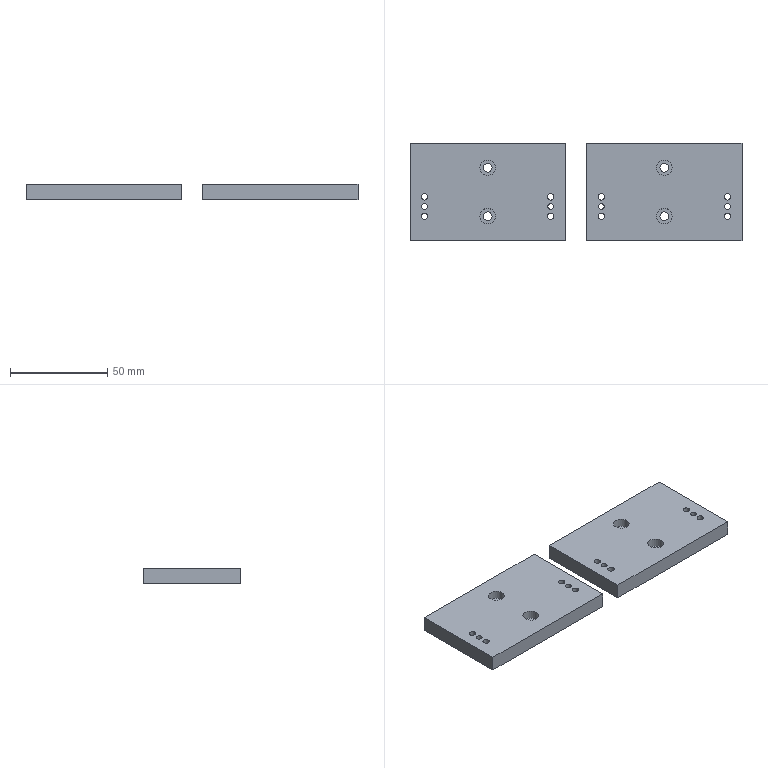Part | NX | 2 solids | 44 faces | box 171 x 50 x 8 mm | volume 62014 mm3 | cylinder 24 | plane 20 | commonest cylinder face diameters 3.3 x8 3 x4 4.5 x4 6 x4 8 x4
STEP:
#1=CARTESIAN_POINT('',(93.25,12.5,2.));
#2=VERTEX_POINT('',#1);
#3=CARTESIAN_POINT('',(91.,12.5,2.));
#4=DIRECTION('',(0.,0.,-1.));
#5=DIRECTION('',(1.,0.,0.));
#6=AXIS2_PLACEMENT_3D('',#3,#4,#5);
#7=CIRCLE('',#6,2.25);
#8=EDGE_CURVE('',#2,#2,#7,.T.);
#9=ORIENTED_EDGE('',*,*,#8,.F.);
#10=EDGE_LOOP('',(#9));
#11=FACE_BOUND('',#10,.T.);
#12=CARTESIAN_POINT('',(94.,12.5,2.));
#13=VERTEX_POINT('',#12);
#14=CARTESIAN_POINT('',(91.,12.5,2.));
#15=DIRECTION('',(0.,0.,-1.));
#16=DIRECTION('',(1.,0.,0.));
#17=AXIS2_PLACEMENT_3D('',#14,#15,#16);
#18=CIRCLE('',#17,3.);
#19=EDGE_CURVE('',#13,#13,#18,.T.);
#20=ORIENTED_EDGE('',*,*,#19,.T.);
#21=EDGE_LOOP('',(#20));
#22=FACE_BOUND('',#21,.T.);
#23=CARTESIAN_POINT('',(91.,37.5,2.));
#24=DIRECTION('',(0.,0.,1.));
#25=DIRECTION('',(1.,0.,0.));
#26=AXIS2_PLACEMENT_3D('',#23,#24,#25);
#27=PLANE('',#26);
#28=ADVANCED_FACE('',(#11,#22),#27,.F.);
#29=CARTESIAN_POINT('',(93.25,37.5,2.));
#30=VERTEX_POINT('',#29);
#31=CARTESIAN_POINT('',(91.,37.5,2.));
#32=DIRECTION('',(0.,0.,-1.));
#33=DIRECTION('',(1.,0.,0.));
#34=AXIS2_PLACEMENT_3D('',#31,#32,#33);
#35=CIRCLE('',#34,2.25);
#36=EDGE_CURVE('',#30,#30,#35,.T.);
#37=ORIENTED_EDGE('',*,*,#36,.F.);
#38=EDGE_LOOP('',(#37));
#39=FACE_BOUND('',#38,.T.);
#40=CARTESIAN_POINT('',(88.,37.5,2.));
#41=VERTEX_POINT('',#40);
#42=CARTESIAN_POINT('',(91.,37.5,2.));
#43=DIRECTION('',(0.,0.,-1.));
#44=DIRECTION('',(-1.,0.,0.));
#45=AXIS2_PLACEMENT_3D('',#42,#43,#44);
#46=CIRCLE('',#45,3.);
#47=EDGE_CURVE('',#41,#41,#46,.T.);
#48=ORIENTED_EDGE('',*,*,#47,.T.);
#49=EDGE_LOOP('',(#48));
#50=FACE_BOUND('',#49,.T.);
#51=CARTESIAN_POINT('',(91.,37.5,2.));
#52=DIRECTION('',(0.,0.,1.));
#53=DIRECTION('',(1.,0.,0.));
#54=AXIS2_PLACEMENT_3D('',#51,#52,#53);
#55=PLANE('',#54);
#56=ADVANCED_FACE('',(#39,#50),#55,.F.);
#57=CARTESIAN_POINT('',(95.,37.5,3.6));
#58=VERTEX_POINT('',#57);
#59=CARTESIAN_POINT('',(91.,37.5,3.6));
#60=DIRECTION('',(0.,0.,1.));
#61=DIRECTION('',(1.,0.,0.));
#62=AXIS2_PLACEMENT_3D('',#59,#60,#61);
#63=CIRCLE('',#62,4.);
#64=EDGE_CURVE('',#58,#58,#63,.T.);
#65=ORIENTED_EDGE('',*,*,#64,.T.);
#66=EDGE_LOOP('',(#65));
#67=FACE_BOUND('',#66,.T.);
#68=CARTESIAN_POINT('',(93.25,37.5,3.6));
#69=VERTEX_POINT('',#68);
#70=CARTESIAN_POINT('',(91.,37.5,3.6));
#71=DIRECTION('',(0.,0.,1.));
#72=DIRECTION('',(1.,0.,0.));
#73=AXIS2_PLACEMENT_3D('',#70,#71,#72);
#74=CIRCLE('',#73,2.25);
#75=EDGE_CURVE('',#69,#69,#74,.T.);
#76=ORIENTED_EDGE('',*,*,#75,.F.);
#77=EDGE_LOOP('',(#76));
#78=FACE_BOUND('',#77,.T.);
#79=CARTESIAN_POINT('',(93.25,37.5,3.6));
#80=DIRECTION('',(0.,0.,-1.));
#81=DIRECTION('',(-1.,0.,0.));
#82=AXIS2_PLACEMENT_3D('',#79,#80,#81);
#83=PLANE('',#82);
#84=ADVANCED_FACE('',(#67,#78),#83,.F.);
#85=CARTESIAN_POINT('',(87.,12.5,3.6));
#86=VERTEX_POINT('',#85);
#87=CARTESIAN_POINT('',(91.,12.5,3.6));
#88=DIRECTION('',(0.,0.,1.));
#89=DIRECTION('',(-1.,0.,0.));
#90=AXIS2_PLACEMENT_3D('',#87,#88,#89);
#91=CIRCLE('',#90,4.);
#92=EDGE_CURVE('',#86,#86,#91,.T.);
#93=ORIENTED_EDGE('',*,*,#92,.T.);
#94=EDGE_LOOP('',(#93));
#95=FACE_BOUND('',#94,.T.);
#96=CARTESIAN_POINT('',(88.75,12.5,3.6));
#97=VERTEX_POINT('',#96);
#98=CARTESIAN_POINT('',(91.,12.5,3.6));
#99=DIRECTION('',(0.,0.,1.));
#100=DIRECTION('',(-1.,0.,0.));
#101=AXIS2_PLACEMENT_3D('',#98,#99,#100);
#102=CIRCLE('',#101,2.25);
#103=EDGE_CURVE('',#97,#97,#102,.T.);
#104=ORIENTED_EDGE('',*,*,#103,.F.);
#105=EDGE_LOOP('',(#104));
#106=FACE_BOUND('',#105,.T.);
#107=CARTESIAN_POINT('',(93.25,37.5,3.6));
#108=DIRECTION('',(0.,0.,-1.));
#109=DIRECTION('',(-1.,0.,0.));
#110=AXIS2_PLACEMENT_3D('',#107,#108,#109);
#111=PLANE('',#110);
#112=ADVANCED_FACE('',(#95,#106),#111,.F.);
#113=CARTESIAN_POINT('',(51.,50.,0.));
#114=VERTEX_POINT('',#113);
#115=CARTESIAN_POINT('',(51.,0.,0.));
#116=VERTEX_POINT('',#115);
#117=CARTESIAN_POINT('',(51.,0.,0.));
#118=DIRECTION('',(0.,-1.,0.));
#119=VECTOR('',#118,1000.);
#120=LINE('',#117,#119);
#121=EDGE_CURVE('',#114,#116,#120,.T.);
#122=ORIENTED_EDGE('',*,*,#121,.F.);
#123=CARTESIAN_POINT('',(131.,50.,0.));
#124=VERTEX_POINT('',#123);
#125=CARTESIAN_POINT('',(51.,50.,0.));
#126=DIRECTION('',(-1.,0.,0.));
#127=VECTOR('',#126,1000.);
#128=LINE('',#125,#127);
#129=EDGE_CURVE('',#124,#114,#128,.T.);
#130=ORIENTED_EDGE('',*,*,#129,.F.);
#131=CARTESIAN_POINT('',(131.,0.,0.));
#132=VERTEX_POINT('',#131);
#133=CARTESIAN_POINT('',(131.,0.,0.));
#134=DIRECTION('',(0.,1.,0.));
#135=VECTOR('',#134,1000.);
#136=LINE('',#133,#135);
#137=EDGE_CURVE('',#132,#124,#136,.T.);
#138=ORIENTED_EDGE('',*,*,#137,.F.);
#139=CARTESIAN_POINT('',(51.,0.,0.));
#140=DIRECTION('',(1.,0.,0.));
#141=VECTOR('',#140,1000.);
#142=LINE('',#139,#141);
#143=EDGE_CURVE('',#116,#132,#142,.T.);
#144=ORIENTED_EDGE('',*,*,#143,.F.);
#145=EDGE_LOOP('',(#122,#130,#138,#144));
#146=FACE_BOUND('',#145,.T.);
#147=CARTESIAN_POINT('',(125.15,12.5,0.));
#148=VERTEX_POINT('',#147);
#149=CARTESIAN_POINT('',(123.5,12.5,0.));
#150=DIRECTION('',(0.,0.,1.));
#151=DIRECTION('',(1.,0.,0.));
#152=AXIS2_PLACEMENT_3D('',#149,#150,#151);
#153=CIRCLE('',#152,1.65);
#154=EDGE_CURVE('',#148,#148,#153,.T.);
#155=ORIENTED_EDGE('',*,*,#154,.T.);
#156=EDGE_LOOP('',(#155));
#157=FACE_BOUND('',#156,.T.);
#158=CARTESIAN_POINT('',(125.15,22.5,0.));
#159=VERTEX_POINT('',#158);
#160=CARTESIAN_POINT('',(123.5,22.5,0.));
#161=DIRECTION('',(0.,0.,1.));
#162=DIRECTION('',(1.,0.,0.));
#163=AXIS2_PLACEMENT_3D('',#160,#161,#162);
#164=CIRCLE('',#163,1.65);
#165=EDGE_CURVE('',#159,#159,#164,.T.);
#166=ORIENTED_EDGE('',*,*,#165,.T.);
#167=EDGE_LOOP('',(#166));
#168=FACE_BOUND('',#167,.T.);
#169=CARTESIAN_POINT('',(60.15,12.5,0.));
#170=VERTEX_POINT('',#169);
#171=CARTESIAN_POINT('',(58.5,12.5,0.));
#172=DIRECTION('',(0.,0.,1.));
#173=DIRECTION('',(1.,0.,0.));
#174=AXIS2_PLACEMENT_3D('',#171,#172,#173);
#175=CIRCLE('',#174,1.65);
#176=EDGE_CURVE('',#170,#170,#175,.T.);
#177=ORIENTED_EDGE('',*,*,#176,.T.);
#178=EDGE_LOOP('',(#177));
#179=FACE_BOUND('',#178,.T.);
#180=CARTESIAN_POINT('',(60.15,22.5,0.));
#181=VERTEX_POINT('',#180);
#182=CARTESIAN_POINT('',(58.5,22.5,0.));
#183=DIRECTION('',(0.,0.,1.));
#184=DIRECTION('',(1.,0.,0.));
#185=AXIS2_PLACEMENT_3D('',#182,#183,#184);
#186=CIRCLE('',#185,1.65);
#187=EDGE_CURVE('',#181,#181,#186,.T.);
#188=ORIENTED_EDGE('',*,*,#187,.T.);
#189=EDGE_LOOP('',(#188));
#190=FACE_BOUND('',#189,.T.);
#191=CARTESIAN_POINT('',(125.,17.5,0.));
#192=VERTEX_POINT('',#191);
#193=CARTESIAN_POINT('',(123.5,17.5,0.));
#194=DIRECTION('',(0.,0.,1.));
#195=DIRECTION('',(1.,0.,0.));
#196=AXIS2_PLACEMENT_3D('',#193,#194,#195);
#197=CIRCLE('',#196,1.5);
#198=EDGE_CURVE('',#192,#192,#197,.T.);
#199=ORIENTED_EDGE('',*,*,#198,.T.);
#200=EDGE_LOOP('',(#199));
#201=FACE_BOUND('',#200,.T.);
#202=CARTESIAN_POINT('',(60.,17.5,0.));
#203=VERTEX_POINT('',#202);
#204=CARTESIAN_POINT('',(58.5,17.5,0.));
#205=DIRECTION('',(0.,0.,1.));
#206=DIRECTION('',(1.,0.,0.));
#207=AXIS2_PLACEMENT_3D('',#204,#205,#206);
#208=CIRCLE('',#207,1.5);
#209=EDGE_CURVE('',#203,#203,#208,.T.);
#210=ORIENTED_EDGE('',*,*,#209,.T.);
#211=EDGE_LOOP('',(#210));
#212=FACE_BOUND('',#211,.T.);
#213=CARTESIAN_POINT('',(88.,37.5,0.));
#214=VERTEX_POINT('',#213);
#215=CARTESIAN_POINT('',(91.,37.5,0.));
#216=DIRECTION('',(0.,0.,-1.));
#217=DIRECTION('',(-1.,0.,0.));
#218=AXIS2_PLACEMENT_3D('',#215,#216,#217);
#219=CIRCLE('',#218,3.);
#220=EDGE_CURVE('',#214,#214,#219,.T.);
#221=ORIENTED_EDGE('',*,*,#220,.F.);
#222=EDGE_LOOP('',(#221));
#223=FACE_BOUND('',#222,.T.);
#224=CARTESIAN_POINT('',(88.,12.5,0.));
#225=VERTEX_POINT('',#224);
#226=CARTESIAN_POINT('',(91.,12.5,0.));
#227=DIRECTION('',(0.,0.,-1.));
#228=DIRECTION('',(-1.,0.,0.));
#229=AXIS2_PLACEMENT_3D('',#226,#227,#228);
#230=CIRCLE('',#229,3.);
#231=EDGE_CURVE('',#225,#225,#230,.T.);
#232=ORIENTED_EDGE('',*,*,#231,.F.);
#233=EDGE_LOOP('',(#232));
#234=FACE_BOUND('',#233,.T.);
#235=CARTESIAN_POINT('',(91.,0.,0.));
#236=DIRECTION('',(0.,0.,-1.));
#237=DIRECTION('',(-1.,0.,0.));
#238=AXIS2_PLACEMENT_3D('',#235,#236,#237);
#239=PLANE('',#238);
#240=ADVANCED_FACE('',(#146,#157,#168,#179,#190,#201,#212,#223,#234),#239,.T.);
#241=CARTESIAN_POINT('',(51.,50.,8.));
#242=VERTEX_POINT('',#241);
#243=CARTESIAN_POINT('',(51.,0.,8.));
#244=VERTEX_POINT('',#243);
#245=CARTESIAN_POINT('',(51.,0.,8.));
#246=DIRECTION('',(0.,-1.,0.));
#247=VECTOR('',#246,1000.);
#248=LINE('',#245,#247);
#249=EDGE_CURVE('',#242,#244,#248,.T.);
#250=ORIENTED_EDGE('',*,*,#249,.T.);
#251=CARTESIAN_POINT('',(131.,0.,8.));
#252=VERTEX_POINT('',#251);
#253=CARTESIAN_POINT('',(51.,0.,8.));
#254=DIRECTION('',(1.,0.,0.));
#255=VECTOR('',#254,1000.);
#256=LINE('',#253,#255);
#257=EDGE_CURVE('',#244,#252,#256,.T.);
#258=ORIENTED_EDGE('',*,*,#257,.T.);
#259=CARTESIAN_POINT('',(131.,50.,8.));
#260=VERTEX_POINT('',#259);
#261=CARTESIAN_POINT('',(131.,0.,8.));
#262=DIRECTION('',(0.,1.,0.));
#263=VECTOR('',#262,1000.);
#264=LINE('',#261,#263);
#265=EDGE_CURVE('',#252,#260,#264,.T.);
#266=ORIENTED_EDGE('',*,*,#265,.T.);
#267=CARTESIAN_POINT('',(51.,50.,8.));
#268=DIRECTION('',(-1.,0.,0.));
#269=VECTOR('',#268,1000.);
#270=LINE('',#267,#269);
#271=EDGE_CURVE('',#260,#242,#270,.T.);
#272=ORIENTED_EDGE('',*,*,#271,.T.);
#273=EDGE_LOOP('',(#250,#258,#266,#272));
#274=FACE_BOUND('',#273,.T.);
#275=CARTESIAN_POINT('',(125.15,12.5,8.));
#276=VERTEX_POINT('',#275);
#277=CARTESIAN_POINT('',(123.5,12.5,8.));
#278=DIRECTION('',(0.,0.,1.));
#279=DIRECTION('',(1.,0.,0.));
#280=AXIS2_PLACEMENT_3D('',#277,#278,#279);
#281=CIRCLE('',#280,1.65);
#282=EDGE_CURVE('',#276,#276,#281,.T.);
#283=ORIENTED_EDGE('',*,*,#282,.F.);
#284=EDGE_LOOP('',(#283));
#285=FACE_BOUND('',#284,.T.);
#286=CARTESIAN_POINT('',(125.15,22.5,8.));
#287=VERTEX_POINT('',#286);
#288=CARTESIAN_POINT('',(123.5,22.5,8.));
#289=DIRECTION('',(0.,0.,1.));
#290=DIRECTION('',(1.,0.,0.));
#291=AXIS2_PLACEMENT_3D('',#288,#289,#290);
#292=CIRCLE('',#291,1.65);
#293=EDGE_CURVE('',#287,#287,#292,.T.);
#294=ORIENTED_EDGE('',*,*,#293,.F.);
#295=EDGE_LOOP('',(#294));
#296=FACE_BOUND('',#295,.T.);
#297=CARTESIAN_POINT('',(60.15,12.5,8.));
#298=VERTEX_POINT('',#297);
#299=CARTESIAN_POINT('',(58.5,12.5,8.));
#300=DIRECTION('',(0.,0.,1.));
#301=DIRECTION('',(1.,0.,0.));
#302=AXIS2_PLACEMENT_3D('',#299,#300,#301);
#303=CIRCLE('',#302,1.65);
#304=EDGE_CURVE('',#298,#298,#303,.T.);
#305=ORIENTED_EDGE('',*,*,#304,.F.);
#306=EDGE_LOOP('',(#305));
#307=FACE_BOUND('',#306,.T.);
#308=CARTESIAN_POINT('',(60.15,22.5,8.));
#309=VERTEX_POINT('',#308);
#310=CARTESIAN_POINT('',(58.5,22.5,8.));
#311=DIRECTION('',(0.,0.,1.));
#312=DIRECTION('',(1.,0.,0.));
#313=AXIS2_PLACEMENT_3D('',#310,#311,#312);
#314=CIRCLE('',#313,1.65);
#315=EDGE_CURVE('',#309,#309,#314,.T.);
#316=ORIENTED_EDGE('',*,*,#315,.F.);
#317=EDGE_LOOP('',(#316));
#318=FACE_BOUND('',#317,.T.);
#319=CARTESIAN_POINT('',(125.,17.5,8.));
#320=VERTEX_POINT('',#319);
#321=CARTESIAN_POINT('',(123.5,17.5,8.));
#322=DIRECTION('',(0.,0.,1.));
#323=DIRECTION('',(1.,0.,0.));
#324=AXIS2_PLACEMENT_3D('',#321,#322,#323);
#325=CIRCLE('',#324,1.5);
#326=EDGE_CURVE('',#320,#320,#325,.T.);
#327=ORIENTED_EDGE('',*,*,#326,.F.);
#328=EDGE_LOOP('',(#327));
#329=FACE_BOUND('',#328,.T.);
#330=CARTESIAN_POINT('',(60.,17.5,8.));
#331=VERTEX_POINT('',#330);
#332=CARTESIAN_POINT('',(58.5,17.5,8.));
#333=DIRECTION('',(0.,0.,1.));
#334=DIRECTION('',(1.,0.,0.));
#335=AXIS2_PLACEMENT_3D('',#332,#333,#334);
#336=CIRCLE('',#335,1.5);
#337=EDGE_CURVE('',#331,#331,#336,.T.);
#338=ORIENTED_EDGE('',*,*,#337,.F.);
#339=EDGE_LOOP('',(#338));
#340=FACE_BOUND('',#339,.T.);
#341=CARTESIAN_POINT('',(95.,12.5,8.));
#342=VERTEX_POINT('',#341);
#343=CARTESIAN_POINT('',(91.,12.5,8.));
#344=DIRECTION('',(0.,0.,1.));
#345=DIRECTION('',(1.,0.,0.));
#346=AXIS2_PLACEMENT_3D('',#343,#344,#345);
#347=CIRCLE('',#346,4.);
#348=EDGE_CURVE('',#342,#342,#347,.T.);
#349=ORIENTED_EDGE('',*,*,#348,.F.);
#350=EDGE_LOOP('',(#349));
#351=FACE_BOUND('',#350,.T.);
#352=CARTESIAN_POINT('',(95.,37.5,8.));
#353=VERTEX_POINT('',#352);
#354=CARTESIAN_POINT('',(91.,37.5,8.));
#355=DIRECTION('',(0.,0.,1.));
#356=DIRECTION('',(1.,0.,0.));
#357=AXIS2_PLACEMENT_3D('',#354,#355,#356);
#358=CIRCLE('',#357,4.);
#359=EDGE_CURVE('',#353,#353,#358,.T.);
#360=ORIENTED_EDGE('',*,*,#359,.F.);
#361=EDGE_LOOP('',(#360));
#362=FACE_BOUND('',#361,.T.);
#363=CARTESIAN_POINT('',(91.,0.,8.));
#364=DIRECTION('',(0.,0.,-1.));
#365=DIRECTION('',(-1.,0.,0.));
#366=AXIS2_PLACEMENT_3D('',#363,#364,#365);
#367=PLANE('',#366);
#368=ADVANCED_FACE('',(#274,#285,#296,#307,#318,#329,#340,#351,#362),#367,.F.);
#369=ORIENTED_EDGE('',*,*,#129,.T.);
#370=CARTESIAN_POINT('',(51.,50.,8.));
#371=DIRECTION('',(0.,0.,-1.));
#372=VECTOR('',#371,1000.);
#373=LINE('',#370,#372);
#374=EDGE_CURVE('',#242,#114,#373,.T.);
#375=ORIENTED_EDGE('',*,*,#374,.F.);
#376=ORIENTED_EDGE('',*,*,#271,.F.);
#377=CARTESIAN_POINT('',(131.,50.,8.));
#378=DIRECTION('',(0.,0.,-1.));
#379=VECTOR('',#378,1000.);
#380=LINE('',#377,#379);
#381=EDGE_CURVE('',#260,#124,#380,.T.);
#382=ORIENTED_EDGE('',*,*,#381,.T.);
#383=EDGE_LOOP('',(#369,#375,#376,#382));
#384=FACE_BOUND('',#383,.T.);
#385=CARTESIAN_POINT('',(51.,50.,8.));
#386=DIRECTION('',(0.,-1.,0.));
#387=DIRECTION('',(0.,0.,-1.));
#388=AXIS2_PLACEMENT_3D('',#385,#386,#387);
#389=PLANE('',#388);
#390=ADVANCED_FACE('',(#384),#389,.F.);
#391=ORIENTED_EDGE('',*,*,#137,.T.);
#392=ORIENTED_EDGE('',*,*,#381,.F.);
#393=ORIENTED_EDGE('',*,*,#265,.F.);
#394=CARTESIAN_POINT('',(131.,0.,8.));
#395=DIRECTION('',(0.,0.,-1.));
#396=VECTOR('',#395,1000.);
#397=LINE('',#394,#396);
#398=EDGE_CURVE('',#252,#132,#397,.T.);
#399=ORIENTED_EDGE('',*,*,#398,.T.);
#400=EDGE_LOOP('',(#391,#392,#393,#399));
#401=FACE_BOUND('',#400,.T.);
#402=CARTESIAN_POINT('',(131.,0.,8.));
#403=DIRECTION('',(-1.,0.,0.));
#404=DIRECTION('',(0.,0.,1.));
#405=AXIS2_PLACEMENT_3D('',#402,#403,#404);
#406=PLANE('',#405);
#407=ADVANCED_FACE('',(#401),#406,.F.);
#408=ORIENTED_EDGE('',*,*,#143,.T.);
#409=ORIENTED_EDGE('',*,*,#398,.F.);
#410=ORIENTED_EDGE('',*,*,#257,.F.);
#411=CARTESIAN_POINT('',(51.,0.,8.));
#412=DIRECTION('',(0.,0.,-1.));
#413=VECTOR('',#412,1000.);
#414=LINE('',#411,#413);
#415=EDGE_CURVE('',#244,#116,#414,.T.);
#416=ORIENTED_EDGE('',*,*,#415,.T.);
#417=EDGE_LOOP('',(#408,#409,#410,#416));
#418=FACE_BOUND('',#417,.T.);
#419=CARTESIAN_POINT('',(51.,0.,8.));
#420=DIRECTION('',(0.,1.,0.));
#421=DIRECTION('',(0.,0.,1.));
#422=AXIS2_PLACEMENT_3D('',#419,#420,#421);
#423=PLANE('',#422);
#424=ADVANCED_FACE('',(#418),#423,.F.);
#425=ORIENTED_EDGE('',*,*,#121,.T.);
#426=ORIENTED_EDGE('',*,*,#415,.F.);
#427=ORIENTED_EDGE('',*,*,#249,.F.);
#428=ORIENTED_EDGE('',*,*,#374,.T.);
#429=EDGE_LOOP('',(#425,#426,#427,#428));
#430=FACE_BOUND('',#429,.T.);
#431=CARTESIAN_POINT('',(51.,0.,8.));
#432=DIRECTION('',(1.,0.,0.));
#433=DIRECTION('',(0.,0.,-1.));
#434=AXIS2_PLACEMENT_3D('',#431,#432,#433);
#435=PLANE('',#434);
#436=ADVANCED_FACE('',(#430),#435,.F.);
#437=ORIENTED_EDGE('',*,*,#154,.F.);
#438=EDGE_LOOP('',(#437));
#439=FACE_BOUND('',#438,.T.);
#440=ORIENTED_EDGE('',*,*,#282,.T.);
#441=EDGE_LOOP('',(#440));
#442=FACE_BOUND('',#441,.T.);
#443=CARTESIAN_POINT('',(123.5,12.5,8.));
#444=DIRECTION('',(0.,0.,1.));
#445=DIRECTION('',(1.,0.,0.));
#446=AXIS2_PLACEMENT_3D('',#443,#444,#445);
#447=CYLINDRICAL_SURFACE('',#446,1.65);
#448=ADVANCED_FACE('',(#439,#442),#447,.F.);
#449=ORIENTED_EDGE('',*,*,#165,.F.);
#450=EDGE_LOOP('',(#449));
#451=FACE_BOUND('',#450,.T.);
#452=ORIENTED_EDGE('',*,*,#293,.T.);
#453=EDGE_LOOP('',(#452));
#454=FACE_BOUND('',#453,.T.);
#455=CARTESIAN_POINT('',(123.5,22.5,8.));
#456=DIRECTION('',(0.,0.,1.));
#457=DIRECTION('',(1.,0.,0.));
#458=AXIS2_PLACEMENT_3D('',#455,#456,#457);
#459=CYLINDRICAL_SURFACE('',#458,1.65);
#460=ADVANCED_FACE('',(#451,#454),#459,.F.);
#461=ORIENTED_EDGE('',*,*,#176,.F.);
#462=EDGE_LOOP('',(#461));
#463=FACE_BOUND('',#462,.T.);
#464=ORIENTED_EDGE('',*,*,#304,.T.);
#465=EDGE_LOOP('',(#464));
#466=FACE_BOUND('',#465,.T.);
#467=CARTESIAN_POINT('',(58.5,12.5,8.));
#468=DIRECTION('',(0.,0.,1.));
#469=DIRECTION('',(1.,0.,0.));
#470=AXIS2_PLACEMENT_3D('',#467,#468,#469);
#471=CYLINDRICAL_SURFACE('',#470,1.65);
#472=ADVANCED_FACE('',(#463,#466),#471,.F.);
#473=ORIENTED_EDGE('',*,*,#187,.F.);
#474=EDGE_LOOP('',(#473));
#475=FACE_BOUND('',#474,.T.);
#476=ORIENTED_EDGE('',*,*,#315,.T.);
#477=EDGE_LOOP('',(#476));
#478=FACE_BOUND('',#477,.T.);
#479=CARTESIAN_POINT('',(58.5,22.5,8.));
#480=DIRECTION('',(0.,0.,1.));
#481=DIRECTION('',(1.,0.,0.));
#482=AXIS2_PLACEMENT_3D('',#479,#480,#481);
#483=CYLINDRICAL_SURFACE('',#482,1.65);
#484=ADVANCED_FACE('',(#475,#478),#483,.F.);
#485=ORIENTED_EDGE('',*,*,#198,.F.);
#486=EDGE_LOOP('',(#485));
#487=FACE_BOUND('',#486,.T.);
#488=ORIENTED_EDGE('',*,*,#326,.T.);
#489=EDGE_LOOP('',(#488));
#490=FACE_BOUND('',#489,.T.);
#491=CARTESIAN_POINT('',(123.5,17.5,8.));
#492=DIRECTION('',(0.,0.,1.));
#493=DIRECTION('',(1.,0.,0.));
#494=AXIS2_PLACEMENT_3D('',#491,#492,#493);
#495=CYLINDRICAL_SURFACE('',#494,1.5);
#496=ADVANCED_FACE('',(#487,#490),#495,.F.);
#497=ORIENTED_EDGE('',*,*,#209,.F.);
#498=EDGE_LOOP('',(#497));
#499=FACE_BOUND('',#498,.T.);
#500=ORIENTED_EDGE('',*,*,#337,.T.);
#501=EDGE_LOOP('',(#500));
#502=FACE_BOUND('',#501,.T.);
#503=CARTESIAN_POINT('',(58.5,17.5,8.));
#504=DIRECTION('',(0.,0.,1.));
#505=DIRECTION('',(1.,0.,0.));
#506=AXIS2_PLACEMENT_3D('',#503,#504,#505);
#507=CYLINDRICAL_SURFACE('',#506,1.5);
#508=ADVANCED_FACE('',(#499,#502),#507,.F.);
#509=ORIENTED_EDGE('',*,*,#8,.T.);
#510=EDGE_LOOP('',(#509));
#511=FACE_BOUND('',#510,.T.);
#512=ORIENTED_EDGE('',*,*,#103,.T.);
#513=EDGE_LOOP('',(#512));
#514=FACE_BOUND('',#513,.T.);
#515=CARTESIAN_POINT('',(91.,12.5,8.));
#516=DIRECTION('',(0.,0.,1.));
#517=DIRECTION('',(1.,0.,0.));
#518=AXIS2_PLACEMENT_3D('',#515,#516,#517);
#519=CYLINDRICAL_SURFACE('',#518,2.25);
#520=ADVANCED_FACE('',(#511,#514),#519,.F.);
#521=ORIENTED_EDGE('',*,*,#92,.F.);
#522=EDGE_LOOP('',(#521));
#523=FACE_BOUND('',#522,.T.);
#524=ORIENTED_EDGE('',*,*,#348,.T.);
#525=EDGE_LOOP('',(#524));
#526=FACE_BOUND('',#525,.T.);
#527=CARTESIAN_POINT('',(91.,12.5,8.));
#528=DIRECTION('',(0.,0.,1.));
#529=DIRECTION('',(1.,0.,0.));
#530=AXIS2_PLACEMENT_3D('',#527,#528,#529);
#531=CYLINDRICAL_SURFACE('',#530,4.);
#532=ADVANCED_FACE('',(#523,#526),#531,.F.);
#533=ORIENTED_EDGE('',*,*,#36,.T.);
#534=EDGE_LOOP('',(#533));
#535=FACE_BOUND('',#534,.T.);
#536=ORIENTED_EDGE('',*,*,#75,.T.);
#537=EDGE_LOOP('',(#536));
#538=FACE_BOUND('',#537,.T.);
#539=CARTESIAN_POINT('',(91.,37.5,8.));
#540=DIRECTION('',(0.,0.,1.));
#541=DIRECTION('',(1.,0.,0.));
#542=AXIS2_PLACEMENT_3D('',#539,#540,#541);
#543=CYLINDRICAL_SURFACE('',#542,2.25);
#544=ADVANCED_FACE('',(#535,#538),#543,.F.);
#545=ORIENTED_EDGE('',*,*,#64,.F.);
#546=EDGE_LOOP('',(#545));
#547=FACE_BOUND('',#546,.T.);
#548=ORIENTED_EDGE('',*,*,#359,.T.);
#549=EDGE_LOOP('',(#548));
#550=FACE_BOUND('',#549,.T.);
#551=CARTESIAN_POINT('',(91.,37.5,8.));
#552=DIRECTION('',(0.,0.,1.));
#553=DIRECTION('',(1.,0.,0.));
#554=AXIS2_PLACEMENT_3D('',#551,#552,#553);
#555=CYLINDRICAL_SURFACE('',#554,4.);
#556=ADVANCED_FACE('',(#547,#550),#555,.F.);
#557=ORIENTED_EDGE('',*,*,#220,.T.);
#558=EDGE_LOOP('',(#557));
#559=FACE_BOUND('',#558,.T.);
#560=ORIENTED_EDGE('',*,*,#47,.F.);
#561=EDGE_LOOP('',(#560));
#562=FACE_BOUND('',#561,.T.);
#563=CARTESIAN_POINT('',(91.,37.5,0.));
#564=DIRECTION('',(0.,0.,-1.));
#565=DIRECTION('',(-1.,0.,0.));
#566=AXIS2_PLACEMENT_3D('',#563,#564,#565);
#567=CYLINDRICAL_SURFACE('',#566,3.);
#568=ADVANCED_FACE('',(#559,#562),#567,.F.);
#569=ORIENTED_EDGE('',*,*,#231,.T.);
#570=EDGE_LOOP('',(#569));
#571=FACE_BOUND('',#570,.T.);
#572=ORIENTED_EDGE('',*,*,#19,.F.);
#573=EDGE_LOOP('',(#572));
#574=FACE_BOUND('',#573,.T.);
#575=CARTESIAN_POINT('',(91.,12.5,0.));
#576=DIRECTION('',(0.,0.,-1.));
#577=DIRECTION('',(-1.,0.,0.));
#578=AXIS2_PLACEMENT_3D('',#575,#576,#577);
#579=CYLINDRICAL_SURFACE('',#578,3.);
#580=ADVANCED_FACE('',(#571,#574),#579,.F.);
#581=CLOSED_SHELL('',(#28,#56,#84,#112,#240,#368,#390,#407,#424,#436,#448,#460,#472,#484,#496,#508,#520,#532,#544,#556,#568,#580));
#582=MANIFOLD_SOLID_BREP('',#581);
#583=CARTESIAN_POINT('',(2.25,12.5,2.));
#584=VERTEX_POINT('',#583);
#585=CARTESIAN_POINT('',(0.,12.5,2.));
#586=DIRECTION('',(0.,0.,-1.));
#587=DIRECTION('',(1.,0.,0.));
#588=AXIS2_PLACEMENT_3D('',#585,#586,#587);
#589=CIRCLE('',#588,2.25);
#590=EDGE_CURVE('',#584,#584,#589,.T.);
#591=ORIENTED_EDGE('',*,*,#590,.F.);
#592=EDGE_LOOP('',(#591));
#593=FACE_BOUND('',#592,.T.);
#594=CARTESIAN_POINT('',(3.,12.5,2.));
#595=VERTEX_POINT('',#594);
#596=CARTESIAN_POINT('',(0.,12.5,2.));
#597=DIRECTION('',(0.,0.,-1.));
#598=DIRECTION('',(1.,0.,0.));
#599=AXIS2_PLACEMENT_3D('',#596,#597,#598);
#600=CIRCLE('',#599,3.);
#601=EDGE_CURVE('',#595,#595,#600,.T.);
#602=ORIENTED_EDGE('',*,*,#601,.T.);
#603=EDGE_LOOP('',(#602));
#604=FACE_BOUND('',#603,.T.);
#605=CARTESIAN_POINT('',(0.,37.5,2.));
#606=DIRECTION('',(0.,0.,1.));
#607=DIRECTION('',(1.,0.,0.));
#608=AXIS2_PLACEMENT_3D('',#605,#606,#607);
#609=PLANE('',#608);
#610=ADVANCED_FACE('',(#593,#604),#609,.F.);
#611=CARTESIAN_POINT('',(2.25,37.5,2.));
#612=VERTEX_POINT('',#611);
#613=CARTESIAN_POINT('',(0.,37.5,2.));
#614=DIRECTION('',(0.,0.,-1.));
#615=DIRECTION('',(1.,0.,0.));
#616=AXIS2_PLACEMENT_3D('',#613,#614,#615);
#617=CIRCLE('',#616,2.25);
#618=EDGE_CURVE('',#612,#612,#617,.T.);
#619=ORIENTED_EDGE('',*,*,#618,.F.);
#620=EDGE_LOOP('',(#619));
#621=FACE_BOUND('',#620,.T.);
#622=CARTESIAN_POINT('',(-3.,37.5,2.));
#623=VERTEX_POINT('',#622);
#624=CARTESIAN_POINT('',(0.,37.5,2.));
#625=DIRECTION('',(0.,0.,-1.));
#626=DIRECTION('',(-1.,0.,0.));
#627=AXIS2_PLACEMENT_3D('',#624,#625,#626);
#628=CIRCLE('',#627,3.);
#629=EDGE_CURVE('',#623,#623,#628,.T.);
#630=ORIENTED_EDGE('',*,*,#629,.T.);
#631=EDGE_LOOP('',(#630));
#632=FACE_BOUND('',#631,.T.);
#633=CARTESIAN_POINT('',(0.,37.5,2.));
#634=DIRECTION('',(0.,0.,1.));
#635=DIRECTION('',(1.,0.,0.));
#636=AXIS2_PLACEMENT_3D('',#633,#634,#635);
#637=PLANE('',#636);
#638=ADVANCED_FACE('',(#621,#632),#637,.F.);
#639=CARTESIAN_POINT('',(4.,37.5,3.6));
#640=VERTEX_POINT('',#639);
#641=CARTESIAN_POINT('',(0.,37.5,3.6));
#642=DIRECTION('',(0.,0.,1.));
#643=DIRECTION('',(1.,0.,0.));
#644=AXIS2_PLACEMENT_3D('',#641,#642,#643);
#645=CIRCLE('',#644,4.);
#646=EDGE_CURVE('',#640,#640,#645,.T.);
#647=ORIENTED_EDGE('',*,*,#646,.T.);
#648=EDGE_LOOP('',(#647));
#649=FACE_BOUND('',#648,.T.);
#650=CARTESIAN_POINT('',(2.25,37.5,3.6));
#651=VERTEX_POINT('',#650);
#652=CARTESIAN_POINT('',(0.,37.5,3.6));
#653=DIRECTION('',(0.,0.,1.));
#654=DIRECTION('',(1.,0.,0.));
#655=AXIS2_PLACEMENT_3D('',#652,#653,#654);
#656=CIRCLE('',#655,2.25);
#657=EDGE_CURVE('',#651,#651,#656,.T.);
#658=ORIENTED_EDGE('',*,*,#657,.F.);
#659=EDGE_LOOP('',(#658));
#660=FACE_BOUND('',#659,.T.);
#661=CARTESIAN_POINT('',(2.25,37.5,3.6));
#662=DIRECTION('',(0.,0.,-1.));
#663=DIRECTION('',(-1.,0.,0.));
#664=AXIS2_PLACEMENT_3D('',#661,#662,#663);
#665=PLANE('',#664);
#666=ADVANCED_FACE('',(#649,#660),#665,.F.);
#667=CARTESIAN_POINT('',(-4.,12.5,3.6));
#668=VERTEX_POINT('',#667);
#669=CARTESIAN_POINT('',(0.,12.5,3.6));
#670=DIRECTION('',(0.,0.,1.));
#671=DIRECTION('',(-1.,0.,0.));
#672=AXIS2_PLACEMENT_3D('',#669,#670,#671);
#673=CIRCLE('',#672,4.);
#674=EDGE_CURVE('',#668,#668,#673,.T.);
#675=ORIENTED_EDGE('',*,*,#674,.T.);
#676=EDGE_LOOP('',(#675));
#677=FACE_BOUND('',#676,.T.);
#678=CARTESIAN_POINT('',(-2.25,12.5,3.6));
#679=VERTEX_POINT('',#678);
#680=CARTESIAN_POINT('',(0.,12.5,3.6));
#681=DIRECTION('',(0.,0.,1.));
#682=DIRECTION('',(-1.,0.,0.));
#683=AXIS2_PLACEMENT_3D('',#680,#681,#682);
#684=CIRCLE('',#683,2.25);
#685=EDGE_CURVE('',#679,#679,#684,.T.);
#686=ORIENTED_EDGE('',*,*,#685,.F.);
#687=EDGE_LOOP('',(#686));
#688=FACE_BOUND('',#687,.T.);
#689=CARTESIAN_POINT('',(2.25,37.5,3.6));
#690=DIRECTION('',(0.,0.,-1.));
#691=DIRECTION('',(-1.,0.,0.));
#692=AXIS2_PLACEMENT_3D('',#689,#690,#691);
#693=PLANE('',#692);
#694=ADVANCED_FACE('',(#677,#688),#693,.F.);
#695=CARTESIAN_POINT('',(-40.,50.,0.));
#696=VERTEX_POINT('',#695);
#697=CARTESIAN_POINT('',(-40.,0.,0.));
#698=VERTEX_POINT('',#697);
#699=CARTESIAN_POINT('',(-40.,0.,0.));
#700=DIRECTION('',(0.,-1.,0.));
#701=VECTOR('',#700,1000.);
#702=LINE('',#699,#701);
#703=EDGE_CURVE('',#696,#698,#702,.T.);
#704=ORIENTED_EDGE('',*,*,#703,.F.);
#705=CARTESIAN_POINT('',(40.,50.,0.));
#706=VERTEX_POINT('',#705);
#707=CARTESIAN_POINT('',(-40.,50.,0.));
#708=DIRECTION('',(-1.,0.,0.));
#709=VECTOR('',#708,1000.);
#710=LINE('',#707,#709);
#711=EDGE_CURVE('',#706,#696,#710,.T.);
#712=ORIENTED_EDGE('',*,*,#711,.F.);
#713=CARTESIAN_POINT('',(40.,0.,0.));
#714=VERTEX_POINT('',#713);
#715=CARTESIAN_POINT('',(40.,0.,0.));
#716=DIRECTION('',(0.,1.,0.));
#717=VECTOR('',#716,1000.);
#718=LINE('',#715,#717);
#719=EDGE_CURVE('',#714,#706,#718,.T.);
#720=ORIENTED_EDGE('',*,*,#719,.F.);
#721=CARTESIAN_POINT('',(-40.,0.,0.));
#722=DIRECTION('',(1.,0.,0.));
#723=VECTOR('',#722,1000.);
#724=LINE('',#721,#723);
#725=EDGE_CURVE('',#698,#714,#724,.T.);
#726=ORIENTED_EDGE('',*,*,#725,.F.);
#727=EDGE_LOOP('',(#704,#712,#720,#726));
#728=FACE_BOUND('',#727,.T.);
#729=CARTESIAN_POINT('',(34.15,12.5,0.));
#730=VERTEX_POINT('',#729);
#731=CARTESIAN_POINT('',(32.5,12.5,0.));
#732=DIRECTION('',(0.,0.,1.));
#733=DIRECTION('',(1.,0.,0.));
#734=AXIS2_PLACEMENT_3D('',#731,#732,#733);
#735=CIRCLE('',#734,1.65);
#736=EDGE_CURVE('',#730,#730,#735,.T.);
#737=ORIENTED_EDGE('',*,*,#736,.T.);
#738=EDGE_LOOP('',(#737));
#739=FACE_BOUND('',#738,.T.);
#740=CARTESIAN_POINT('',(34.15,22.5,0.));
#741=VERTEX_POINT('',#740);
#742=CARTESIAN_POINT('',(32.5,22.5,0.));
#743=DIRECTION('',(0.,0.,1.));
#744=DIRECTION('',(1.,0.,0.));
#745=AXIS2_PLACEMENT_3D('',#742,#743,#744);
#746=CIRCLE('',#745,1.65);
#747=EDGE_CURVE('',#741,#741,#746,.T.);
#748=ORIENTED_EDGE('',*,*,#747,.T.);
#749=EDGE_LOOP('',(#748));
#750=FACE_BOUND('',#749,.T.);
#751=CARTESIAN_POINT('',(-30.85,12.5,0.));
#752=VERTEX_POINT('',#751);
#753=CARTESIAN_POINT('',(-32.5,12.5,0.));
#754=DIRECTION('',(0.,0.,1.));
#755=DIRECTION('',(1.,0.,0.));
#756=AXIS2_PLACEMENT_3D('',#753,#754,#755);
#757=CIRCLE('',#756,1.65);
#758=EDGE_CURVE('',#752,#752,#757,.T.);
#759=ORIENTED_EDGE('',*,*,#758,.T.);
#760=EDGE_LOOP('',(#759));
#761=FACE_BOUND('',#760,.T.);
#762=CARTESIAN_POINT('',(-30.85,22.5,0.));
#763=VERTEX_POINT('',#762);
#764=CARTESIAN_POINT('',(-32.5,22.5,0.));
#765=DIRECTION('',(0.,0.,1.));
#766=DIRECTION('',(1.,0.,0.));
#767=AXIS2_PLACEMENT_3D('',#764,#765,#766);
#768=CIRCLE('',#767,1.65);
#769=EDGE_CURVE('',#763,#763,#768,.T.);
#770=ORIENTED_EDGE('',*,*,#769,.T.);
#771=EDGE_LOOP('',(#770));
#772=FACE_BOUND('',#771,.T.);
#773=CARTESIAN_POINT('',(34.,17.5,0.));
#774=VERTEX_POINT('',#773);
#775=CARTESIAN_POINT('',(32.5,17.5,0.));
#776=DIRECTION('',(0.,0.,1.));
#777=DIRECTION('',(1.,0.,0.));
#778=AXIS2_PLACEMENT_3D('',#775,#776,#777);
#779=CIRCLE('',#778,1.5);
#780=EDGE_CURVE('',#774,#774,#779,.T.);
#781=ORIENTED_EDGE('',*,*,#780,.T.);
#782=EDGE_LOOP('',(#781));
#783=FACE_BOUND('',#782,.T.);
#784=CARTESIAN_POINT('',(-31.,17.5,0.));
#785=VERTEX_POINT('',#784);
#786=CARTESIAN_POINT('',(-32.5,17.5,0.));
#787=DIRECTION('',(0.,0.,1.));
#788=DIRECTION('',(1.,0.,0.));
#789=AXIS2_PLACEMENT_3D('',#786,#787,#788);
#790=CIRCLE('',#789,1.5);
#791=EDGE_CURVE('',#785,#785,#790,.T.);
#792=ORIENTED_EDGE('',*,*,#791,.T.);
#793=EDGE_LOOP('',(#792));
#794=FACE_BOUND('',#793,.T.);
#795=CARTESIAN_POINT('',(-3.,37.5,0.));
#796=VERTEX_POINT('',#795);
#797=CARTESIAN_POINT('',(0.,37.5,0.));
#798=DIRECTION('',(0.,0.,-1.));
#799=DIRECTION('',(-1.,0.,0.));
#800=AXIS2_PLACEMENT_3D('',#797,#798,#799);
#801=CIRCLE('',#800,3.);
#802=EDGE_CURVE('',#796,#796,#801,.T.);
#803=ORIENTED_EDGE('',*,*,#802,.F.);
#804=EDGE_LOOP('',(#803));
#805=FACE_BOUND('',#804,.T.);
#806=CARTESIAN_POINT('',(-3.,12.5,0.));
#807=VERTEX_POINT('',#806);
#808=CARTESIAN_POINT('',(0.,12.5,0.));
#809=DIRECTION('',(0.,0.,-1.));
#810=DIRECTION('',(-1.,0.,0.));
#811=AXIS2_PLACEMENT_3D('',#808,#809,#810);
#812=CIRCLE('',#811,3.);
#813=EDGE_CURVE('',#807,#807,#812,.T.);
#814=ORIENTED_EDGE('',*,*,#813,.F.);
#815=EDGE_LOOP('',(#814));
#816=FACE_BOUND('',#815,.T.);
#817=CARTESIAN_POINT('',(0.,0.,0.));
#818=DIRECTION('',(0.,0.,-1.));
#819=DIRECTION('',(-1.,0.,0.));
#820=AXIS2_PLACEMENT_3D('',#817,#818,#819);
#821=PLANE('',#820);
#822=ADVANCED_FACE('',(#728,#739,#750,#761,#772,#783,#794,#805,#816),#821,.T.);
#823=CARTESIAN_POINT('',(-40.,50.,8.));
#824=VERTEX_POINT('',#823);
#825=CARTESIAN_POINT('',(-40.,0.,8.));
#826=VERTEX_POINT('',#825);
#827=CARTESIAN_POINT('',(-40.,0.,8.));
#828=DIRECTION('',(0.,-1.,0.));
#829=VECTOR('',#828,1000.);
#830=LINE('',#827,#829);
#831=EDGE_CURVE('',#824,#826,#830,.T.);
#832=ORIENTED_EDGE('',*,*,#831,.T.);
#833=CARTESIAN_POINT('',(40.,0.,8.));
#834=VERTEX_POINT('',#833);
#835=CARTESIAN_POINT('',(-40.,0.,8.));
#836=DIRECTION('',(1.,0.,0.));
#837=VECTOR('',#836,1000.);
#838=LINE('',#835,#837);
#839=EDGE_CURVE('',#826,#834,#838,.T.);
#840=ORIENTED_EDGE('',*,*,#839,.T.);
#841=CARTESIAN_POINT('',(40.,50.,8.));
#842=VERTEX_POINT('',#841);
#843=CARTESIAN_POINT('',(40.,0.,8.));
#844=DIRECTION('',(0.,1.,0.));
#845=VECTOR('',#844,1000.);
#846=LINE('',#843,#845);
#847=EDGE_CURVE('',#834,#842,#846,.T.);
#848=ORIENTED_EDGE('',*,*,#847,.T.);
#849=CARTESIAN_POINT('',(-40.,50.,8.));
#850=DIRECTION('',(-1.,0.,0.));
#851=VECTOR('',#850,1000.);
#852=LINE('',#849,#851);
#853=EDGE_CURVE('',#842,#824,#852,.T.);
#854=ORIENTED_EDGE('',*,*,#853,.T.);
#855=EDGE_LOOP('',(#832,#840,#848,#854));
#856=FACE_BOUND('',#855,.T.);
#857=CARTESIAN_POINT('',(34.15,12.5,8.));
#858=VERTEX_POINT('',#857);
#859=CARTESIAN_POINT('',(32.5,12.5,8.));
#860=DIRECTION('',(0.,0.,1.));
#861=DIRECTION('',(1.,0.,0.));
#862=AXIS2_PLACEMENT_3D('',#859,#860,#861);
#863=CIRCLE('',#862,1.65);
#864=EDGE_CURVE('',#858,#858,#863,.T.);
#865=ORIENTED_EDGE('',*,*,#864,.F.);
#866=EDGE_LOOP('',(#865));
#867=FACE_BOUND('',#866,.T.);
#868=CARTESIAN_POINT('',(34.15,22.5,8.));
#869=VERTEX_POINT('',#868);
#870=CARTESIAN_POINT('',(32.5,22.5,8.));
#871=DIRECTION('',(0.,0.,1.));
#872=DIRECTION('',(1.,0.,0.));
#873=AXIS2_PLACEMENT_3D('',#870,#871,#872);
#874=CIRCLE('',#873,1.65);
#875=EDGE_CURVE('',#869,#869,#874,.T.);
#876=ORIENTED_EDGE('',*,*,#875,.F.);
#877=EDGE_LOOP('',(#876));
#878=FACE_BOUND('',#877,.T.);
#879=CARTESIAN_POINT('',(-30.85,12.5,8.));
#880=VERTEX_POINT('',#879);
#881=CARTESIAN_POINT('',(-32.5,12.5,8.));
#882=DIRECTION('',(0.,0.,1.));
#883=DIRECTION('',(1.,0.,0.));
#884=AXIS2_PLACEMENT_3D('',#881,#882,#883);
#885=CIRCLE('',#884,1.65);
#886=EDGE_CURVE('',#880,#880,#885,.T.);
#887=ORIENTED_EDGE('',*,*,#886,.F.);
#888=EDGE_LOOP('',(#887));
#889=FACE_BOUND('',#888,.T.);
#890=CARTESIAN_POINT('',(-30.85,22.5,8.));
#891=VERTEX_POINT('',#890);
#892=CARTESIAN_POINT('',(-32.5,22.5,8.));
#893=DIRECTION('',(0.,0.,1.));
#894=DIRECTION('',(1.,0.,0.));
#895=AXIS2_PLACEMENT_3D('',#892,#893,#894);
#896=CIRCLE('',#895,1.65);
#897=EDGE_CURVE('',#891,#891,#896,.T.);
#898=ORIENTED_EDGE('',*,*,#897,.F.);
#899=EDGE_LOOP('',(#898));
#900=FACE_BOUND('',#899,.T.);
#901=CARTESIAN_POINT('',(34.,17.5,8.));
#902=VERTEX_POINT('',#901);
#903=CARTESIAN_POINT('',(32.5,17.5,8.));
#904=DIRECTION('',(0.,0.,1.));
#905=DIRECTION('',(1.,0.,0.));
#906=AXIS2_PLACEMENT_3D('',#903,#904,#905);
#907=CIRCLE('',#906,1.5);
#908=EDGE_CURVE('',#902,#902,#907,.T.);
#909=ORIENTED_EDGE('',*,*,#908,.F.);
#910=EDGE_LOOP('',(#909));
#911=FACE_BOUND('',#910,.T.);
#912=CARTESIAN_POINT('',(-31.,17.5,8.));
#913=VERTEX_POINT('',#912);
#914=CARTESIAN_POINT('',(-32.5,17.5,8.));
#915=DIRECTION('',(0.,0.,1.));
#916=DIRECTION('',(1.,0.,0.));
#917=AXIS2_PLACEMENT_3D('',#914,#915,#916);
#918=CIRCLE('',#917,1.5);
#919=EDGE_CURVE('',#913,#913,#918,.T.);
#920=ORIENTED_EDGE('',*,*,#919,.F.);
#921=EDGE_LOOP('',(#920));
#922=FACE_BOUND('',#921,.T.);
#923=CARTESIAN_POINT('',(4.,12.5,8.));
#924=VERTEX_POINT('',#923);
#925=CARTESIAN_POINT('',(0.,12.5,8.));
#926=DIRECTION('',(0.,0.,1.));
#927=DIRECTION('',(1.,0.,0.));
#928=AXIS2_PLACEMENT_3D('',#925,#926,#927);
#929=CIRCLE('',#928,4.);
#930=EDGE_CURVE('',#924,#924,#929,.T.);
#931=ORIENTED_EDGE('',*,*,#930,.F.);
#932=EDGE_LOOP('',(#931));
#933=FACE_BOUND('',#932,.T.);
#934=CARTESIAN_POINT('',(4.,37.5,8.));
#935=VERTEX_POINT('',#934);
#936=CARTESIAN_POINT('',(0.,37.5,8.));
#937=DIRECTION('',(0.,0.,1.));
#938=DIRECTION('',(1.,0.,0.));
#939=AXIS2_PLACEMENT_3D('',#936,#937,#938);
#940=CIRCLE('',#939,4.);
#941=EDGE_CURVE('',#935,#935,#940,.T.);
#942=ORIENTED_EDGE('',*,*,#941,.F.);
#943=EDGE_LOOP('',(#942));
#944=FACE_BOUND('',#943,.T.);
#945=CARTESIAN_POINT('',(0.,0.,8.));
#946=DIRECTION('',(0.,0.,-1.));
#947=DIRECTION('',(-1.,0.,0.));
#948=AXIS2_PLACEMENT_3D('',#945,#946,#947);
#949=PLANE('',#948);
#950=ADVANCED_FACE('',(#856,#867,#878,#889,#900,#911,#922,#933,#944),#949,.F.);
#951=ORIENTED_EDGE('',*,*,#711,.T.);
#952=CARTESIAN_POINT('',(-40.,50.,8.));
#953=DIRECTION('',(0.,0.,-1.));
#954=VECTOR('',#953,1000.);
#955=LINE('',#952,#954);
#956=EDGE_CURVE('',#824,#696,#955,.T.);
#957=ORIENTED_EDGE('',*,*,#956,.F.);
#958=ORIENTED_EDGE('',*,*,#853,.F.);
#959=CARTESIAN_POINT('',(40.,50.,8.));
#960=DIRECTION('',(0.,0.,-1.));
#961=VECTOR('',#960,1000.);
#962=LINE('',#959,#961);
#963=EDGE_CURVE('',#842,#706,#962,.T.);
#964=ORIENTED_EDGE('',*,*,#963,.T.);
#965=EDGE_LOOP('',(#951,#957,#958,#964));
#966=FACE_BOUND('',#965,.T.);
#967=CARTESIAN_POINT('',(-40.,50.,8.));
#968=DIRECTION('',(0.,-1.,0.));
#969=DIRECTION('',(0.,0.,-1.));
#970=AXIS2_PLACEMENT_3D('',#967,#968,#969);
#971=PLANE('',#970);
#972=ADVANCED_FACE('',(#966),#971,.F.);
#973=ORIENTED_EDGE('',*,*,#719,.T.);
#974=ORIENTED_EDGE('',*,*,#963,.F.);
#975=ORIENTED_EDGE('',*,*,#847,.F.);
#976=CARTESIAN_POINT('',(40.,0.,8.));
#977=DIRECTION('',(0.,0.,-1.));
#978=VECTOR('',#977,1000.);
#979=LINE('',#976,#978);
#980=EDGE_CURVE('',#834,#714,#979,.T.);
#981=ORIENTED_EDGE('',*,*,#980,.T.);
#982=EDGE_LOOP('',(#973,#974,#975,#981));
#983=FACE_BOUND('',#982,.T.);
#984=CARTESIAN_POINT('',(40.,0.,8.));
#985=DIRECTION('',(-1.,0.,0.));
#986=DIRECTION('',(0.,0.,1.));
#987=AXIS2_PLACEMENT_3D('',#984,#985,#986);
#988=PLANE('',#987);
#989=ADVANCED_FACE('',(#983),#988,.F.);
#990=ORIENTED_EDGE('',*,*,#725,.T.);
#991=ORIENTED_EDGE('',*,*,#980,.F.);
#992=ORIENTED_EDGE('',*,*,#839,.F.);
#993=CARTESIAN_POINT('',(-40.,0.,8.));
#994=DIRECTION('',(0.,0.,-1.));
#995=VECTOR('',#994,1000.);
#996=LINE('',#993,#995);
#997=EDGE_CURVE('',#826,#698,#996,.T.);
#998=ORIENTED_EDGE('',*,*,#997,.T.);
#999=EDGE_LOOP('',(#990,#991,#992,#998));
#1000=FACE_BOUND('',#999,.T.);
#1001=CARTESIAN_POINT('',(-40.,0.,8.));
#1002=DIRECTION('',(0.,1.,0.));
#1003=DIRECTION('',(0.,0.,1.));
#1004=AXIS2_PLACEMENT_3D('',#1001,#1002,#1003);
#1005=PLANE('',#1004);
#1006=ADVANCED_FACE('',(#1000),#1005,.F.);
#1007=ORIENTED_EDGE('',*,*,#703,.T.);
#1008=ORIENTED_EDGE('',*,*,#997,.F.);
#1009=ORIENTED_EDGE('',*,*,#831,.F.);
#1010=ORIENTED_EDGE('',*,*,#956,.T.);
#1011=EDGE_LOOP('',(#1007,#1008,#1009,#1010));
#1012=FACE_BOUND('',#1011,.T.);
#1013=CARTESIAN_POINT('',(-40.,0.,8.));
#1014=DIRECTION('',(1.,0.,0.));
#1015=DIRECTION('',(0.,0.,-1.));
#1016=AXIS2_PLACEMENT_3D('',#1013,#1014,#1015);
#1017=PLANE('',#1016);
#1018=ADVANCED_FACE('',(#1012),#1017,.F.);
#1019=ORIENTED_EDGE('',*,*,#736,.F.);
#1020=EDGE_LOOP('',(#1019));
#1021=FACE_BOUND('',#1020,.T.);
#1022=ORIENTED_EDGE('',*,*,#864,.T.);
#1023=EDGE_LOOP('',(#1022));
#1024=FACE_BOUND('',#1023,.T.);
#1025=CARTESIAN_POINT('',(32.5,12.5,8.));
#1026=DIRECTION('',(0.,0.,1.));
#1027=DIRECTION('',(1.,0.,0.));
#1028=AXIS2_PLACEMENT_3D('',#1025,#1026,#1027);
#1029=CYLINDRICAL_SURFACE('',#1028,1.65);
#1030=ADVANCED_FACE('',(#1021,#1024),#1029,.F.);
#1031=ORIENTED_EDGE('',*,*,#747,.F.);
#1032=EDGE_LOOP('',(#1031));
#1033=FACE_BOUND('',#1032,.T.);
#1034=ORIENTED_EDGE('',*,*,#875,.T.);
#1035=EDGE_LOOP('',(#1034));
#1036=FACE_BOUND('',#1035,.T.);
#1037=CARTESIAN_POINT('',(32.5,22.5,8.));
#1038=DIRECTION('',(0.,0.,1.));
#1039=DIRECTION('',(1.,0.,0.));
#1040=AXIS2_PLACEMENT_3D('',#1037,#1038,#1039);
#1041=CYLINDRICAL_SURFACE('',#1040,1.65);
#1042=ADVANCED_FACE('',(#1033,#1036),#1041,.F.);
#1043=ORIENTED_EDGE('',*,*,#758,.F.);
#1044=EDGE_LOOP('',(#1043));
#1045=FACE_BOUND('',#1044,.T.);
#1046=ORIENTED_EDGE('',*,*,#886,.T.);
#1047=EDGE_LOOP('',(#1046));
#1048=FACE_BOUND('',#1047,.T.);
#1049=CARTESIAN_POINT('',(-32.5,12.5,8.));
#1050=DIRECTION('',(0.,0.,1.));
#1051=DIRECTION('',(1.,0.,0.));
#1052=AXIS2_PLACEMENT_3D('',#1049,#1050,#1051);
#1053=CYLINDRICAL_SURFACE('',#1052,1.65);
#1054=ADVANCED_FACE('',(#1045,#1048),#1053,.F.);
#1055=ORIENTED_EDGE('',*,*,#769,.F.);
#1056=EDGE_LOOP('',(#1055));
#1057=FACE_BOUND('',#1056,.T.);
#1058=ORIENTED_EDGE('',*,*,#897,.T.);
#1059=EDGE_LOOP('',(#1058));
#1060=FACE_BOUND('',#1059,.T.);
#1061=CARTESIAN_POINT('',(-32.5,22.5,8.));
#1062=DIRECTION('',(0.,0.,1.));
#1063=DIRECTION('',(1.,0.,0.));
#1064=AXIS2_PLACEMENT_3D('',#1061,#1062,#1063);
#1065=CYLINDRICAL_SURFACE('',#1064,1.65);
#1066=ADVANCED_FACE('',(#1057,#1060),#1065,.F.);
#1067=ORIENTED_EDGE('',*,*,#780,.F.);
#1068=EDGE_LOOP('',(#1067));
#1069=FACE_BOUND('',#1068,.T.);
#1070=ORIENTED_EDGE('',*,*,#908,.T.);
#1071=EDGE_LOOP('',(#1070));
#1072=FACE_BOUND('',#1071,.T.);
#1073=CARTESIAN_POINT('',(32.5,17.5,8.));
#1074=DIRECTION('',(0.,0.,1.));
#1075=DIRECTION('',(1.,0.,0.));
#1076=AXIS2_PLACEMENT_3D('',#1073,#1074,#1075);
#1077=CYLINDRICAL_SURFACE('',#1076,1.5);
#1078=ADVANCED_FACE('',(#1069,#1072),#1077,.F.);
#1079=ORIENTED_EDGE('',*,*,#791,.F.);
#1080=EDGE_LOOP('',(#1079));
#1081=FACE_BOUND('',#1080,.T.);
#1082=ORIENTED_EDGE('',*,*,#919,.T.);
#1083=EDGE_LOOP('',(#1082));
#1084=FACE_BOUND('',#1083,.T.);
#1085=CARTESIAN_POINT('',(-32.5,17.5,8.));
#1086=DIRECTION('',(0.,0.,1.));
#1087=DIRECTION('',(1.,0.,0.));
#1088=AXIS2_PLACEMENT_3D('',#1085,#1086,#1087);
#1089=CYLINDRICAL_SURFACE('',#1088,1.5);
#1090=ADVANCED_FACE('',(#1081,#1084),#1089,.F.);
#1091=ORIENTED_EDGE('',*,*,#590,.T.);
#1092=EDGE_LOOP('',(#1091));
#1093=FACE_BOUND('',#1092,.T.);
#1094=ORIENTED_EDGE('',*,*,#685,.T.);
#1095=EDGE_LOOP('',(#1094));
#1096=FACE_BOUND('',#1095,.T.);
#1097=CARTESIAN_POINT('',(0.,12.5,8.));
#1098=DIRECTION('',(0.,0.,1.));
#1099=DIRECTION('',(1.,0.,0.));
#1100=AXIS2_PLACEMENT_3D('',#1097,#1098,#1099);
#1101=CYLINDRICAL_SURFACE('',#1100,2.25);
#1102=ADVANCED_FACE('',(#1093,#1096),#1101,.F.);
#1103=ORIENTED_EDGE('',*,*,#674,.F.);
#1104=EDGE_LOOP('',(#1103));
#1105=FACE_BOUND('',#1104,.T.);
#1106=ORIENTED_EDGE('',*,*,#930,.T.);
#1107=EDGE_LOOP('',(#1106));
#1108=FACE_BOUND('',#1107,.T.);
#1109=CARTESIAN_POINT('',(0.,12.5,8.));
#1110=DIRECTION('',(0.,0.,1.));
#1111=DIRECTION('',(1.,0.,0.));
#1112=AXIS2_PLACEMENT_3D('',#1109,#1110,#1111);
#1113=CYLINDRICAL_SURFACE('',#1112,4.);
#1114=ADVANCED_FACE('',(#1105,#1108),#1113,.F.);
#1115=ORIENTED_EDGE('',*,*,#618,.T.);
#1116=EDGE_LOOP('',(#1115));
#1117=FACE_BOUND('',#1116,.T.);
#1118=ORIENTED_EDGE('',*,*,#657,.T.);
#1119=EDGE_LOOP('',(#1118));
#1120=FACE_BOUND('',#1119,.T.);
#1121=CARTESIAN_POINT('',(0.,37.5,8.));
#1122=DIRECTION('',(0.,0.,1.));
#1123=DIRECTION('',(1.,0.,0.));
#1124=AXIS2_PLACEMENT_3D('',#1121,#1122,#1123);
#1125=CYLINDRICAL_SURFACE('',#1124,2.25);
#1126=ADVANCED_FACE('',(#1117,#1120),#1125,.F.);
#1127=ORIENTED_EDGE('',*,*,#646,.F.);
#1128=EDGE_LOOP('',(#1127));
#1129=FACE_BOUND('',#1128,.T.);
#1130=ORIENTED_EDGE('',*,*,#941,.T.);
#1131=EDGE_LOOP('',(#1130));
#1132=FACE_BOUND('',#1131,.T.);
#1133=CARTESIAN_POINT('',(0.,37.5,8.));
#1134=DIRECTION('',(0.,0.,1.));
#1135=DIRECTION('',(1.,0.,0.));
#1136=AXIS2_PLACEMENT_3D('',#1133,#1134,#1135);
#1137=CYLINDRICAL_SURFACE('',#1136,4.);
#1138=ADVANCED_FACE('',(#1129,#1132),#1137,.F.);
#1139=ORIENTED_EDGE('',*,*,#802,.T.);
#1140=EDGE_LOOP('',(#1139));
#1141=FACE_BOUND('',#1140,.T.);
#1142=ORIENTED_EDGE('',*,*,#629,.F.);
#1143=EDGE_LOOP('',(#1142));
#1144=FACE_BOUND('',#1143,.T.);
#1145=CARTESIAN_POINT('',(0.,37.5,0.));
#1146=DIRECTION('',(0.,0.,-1.));
#1147=DIRECTION('',(-1.,0.,0.));
#1148=AXIS2_PLACEMENT_3D('',#1145,#1146,#1147);
#1149=CYLINDRICAL_SURFACE('',#1148,3.);
#1150=ADVANCED_FACE('',(#1141,#1144),#1149,.F.);
#1151=ORIENTED_EDGE('',*,*,#813,.T.);
#1152=EDGE_LOOP('',(#1151));
#1153=FACE_BOUND('',#1152,.T.);
#1154=ORIENTED_EDGE('',*,*,#601,.F.);
#1155=EDGE_LOOP('',(#1154));
#1156=FACE_BOUND('',#1155,.T.);
#1157=CARTESIAN_POINT('',(0.,12.5,0.));
#1158=DIRECTION('',(0.,0.,-1.));
#1159=DIRECTION('',(-1.,0.,0.));
#1160=AXIS2_PLACEMENT_3D('',#1157,#1158,#1159);
#1161=CYLINDRICAL_SURFACE('',#1160,3.);
#1162=ADVANCED_FACE('',(#1153,#1156),#1161,.F.);
#1163=CLOSED_SHELL('',(#610,#638,#666,#694,#822,#950,#972,#989,#1006,#1018,#1030,#1042,#1054,#1066,#1078,#1090,#1102,#1114,#1126,#1138,#1150,#1162));
#1164=MANIFOLD_SOLID_BREP('',#1163);
#1165=(LENGTH_UNIT()NAMED_UNIT(*)SI_UNIT(.MILLI.,.METRE.));
#1166=UNCERTAINTY_MEASURE_WITH_UNIT(LENGTH_MEASURE(0.00001),#1165,'','');
#1167=(NAMED_UNIT(*)PLANE_ANGLE_UNIT()SI_UNIT($,.RADIAN.));
#1168=(NAMED_UNIT(*)SI_UNIT($,.STERADIAN.)SOLID_ANGLE_UNIT());
#1169=(GEOMETRIC_REPRESENTATION_CONTEXT(3)GLOBAL_UNCERTAINTY_ASSIGNED_CONTEXT((#1166))GLOBAL_UNIT_ASSIGNED_CONTEXT((#1165,#1167,#1168))REPRESENTATION_CONTEXT('',''));
#1170=ADVANCED_BREP_SHAPE_REPRESENTATION('',(#582,#1164),#1169);